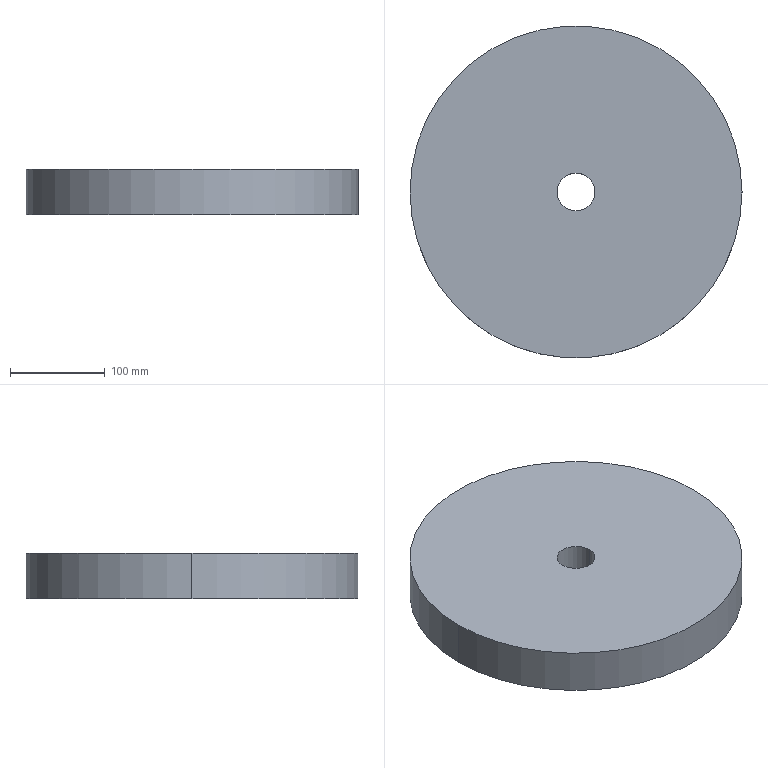Part | STEP file | 1 solid | 6 faces | box 350 x 350 x 48 mm | volume 4557823 mm3 | cylinder 4 | plane 2 | commonest cylinder face diameters 40 x2 350 x2
STEP:
#1=CARTESIAN_POINT('',(0.,0.,0.));
#2=DIRECTION('',(0.,0.,1.));
#3=DIRECTION('',(1.,0.,0.));
#4=AXIS2_PLACEMENT_3D('',#1,#2,#3);
#5=CARTESIAN_POINT('',(175.,0.,0.));
#6=VERTEX_POINT('',#5);
#7=CARTESIAN_POINT('',(-175.,0.,0.));
#8=VERTEX_POINT('',#7);
#9=CARTESIAN_POINT('',(0.,0.,0.));
#10=DIRECTION('',(0.,0.,1.));
#11=DIRECTION('',(1.,0.,0.));
#12=AXIS2_PLACEMENT_3D('',#9,#10,#11);
#13=CIRCLE('',#12,175.);
#14=CARTESIAN_POINT('',(0.,0.,0.));
#15=DIRECTION('',(0.,0.,1.));
#16=DIRECTION('',(1.,0.,0.));
#17=AXIS2_PLACEMENT_3D('',#14,#15,#16);
#18=CYLINDRICAL_SURFACE('',#17,175.);
#19=CARTESIAN_POINT('',(0.,0.));
#20=DIRECTION('',(1.,0.));
#21=VECTOR('',#20,1.);
#22=LINE('',#19,#21);
#23=(GEOMETRIC_REPRESENTATION_CONTEXT(2)PARAMETRIC_REPRESENTATION_CONTEXT()REPRESENTATION_CONTEXT('',''));
#24=DEFINITIONAL_REPRESENTATION('',(#22),#23);
#25=PCURVE('',#18,#24);
#26=CARTESIAN_POINT('',(0.,0.,0.));
#27=DIRECTION('',(0.,0.,1.));
#28=DIRECTION('',(1.,0.,0.));
#29=AXIS2_PLACEMENT_3D('',#26,#27,#28);
#30=PLANE('',#29);
#31=CARTESIAN_POINT('',(0.,0.));
#32=DIRECTION('',(1.,0.));
#33=AXIS2_PLACEMENT_2D('',#31,#32);
#34=CIRCLE('',#33,175.);
#35=(GEOMETRIC_REPRESENTATION_CONTEXT(2)PARAMETRIC_REPRESENTATION_CONTEXT()REPRESENTATION_CONTEXT('',''));
#36=DEFINITIONAL_REPRESENTATION('',(#34),#35);
#37=PCURVE('',#30,#36);
#38=SURFACE_CURVE('',#13,(#25,#37),.PCURVE_S1.);
#39=EDGE_CURVE('',#6,#8,#38,.T.);
#40=ORIENTED_EDGE('',*,*,#39,.T.);
#41=CARTESIAN_POINT('',(-175.,0.,48.));
#42=VERTEX_POINT('',#41);
#43=CARTESIAN_POINT('',(-175.,0.,0.));
#44=DIRECTION('',(0.,0.,1.));
#45=VECTOR('',#44,1.);
#46=LINE('',#43,#45);
#47=CARTESIAN_POINT('',(3.142,0.));
#48=DIRECTION('',(0.,1.));
#49=VECTOR('',#48,1.);
#50=LINE('',#47,#49);
#51=(GEOMETRIC_REPRESENTATION_CONTEXT(2)PARAMETRIC_REPRESENTATION_CONTEXT()REPRESENTATION_CONTEXT('',''));
#52=DEFINITIONAL_REPRESENTATION('',(#50),#51);
#53=PCURVE('',#18,#52);
#54=CARTESIAN_POINT('',(0.,0.,0.));
#55=DIRECTION('',(0.,0.,1.));
#56=DIRECTION('',(1.,0.,0.));
#57=AXIS2_PLACEMENT_3D('',#54,#55,#56);
#58=CYLINDRICAL_SURFACE('',#57,175.);
#59=CARTESIAN_POINT('',(3.142,0.));
#60=DIRECTION('',(0.,1.));
#61=VECTOR('',#60,1.);
#62=LINE('',#59,#61);
#63=(GEOMETRIC_REPRESENTATION_CONTEXT(2)PARAMETRIC_REPRESENTATION_CONTEXT()REPRESENTATION_CONTEXT('',''));
#64=DEFINITIONAL_REPRESENTATION('',(#62),#63);
#65=PCURVE('',#58,#64);
#66=SURFACE_CURVE('',#46,(#53,#65),.PCURVE_S1.);
#67=EDGE_CURVE('',#8,#42,#66,.T.);
#68=ORIENTED_EDGE('',*,*,#67,.T.);
#69=CARTESIAN_POINT('',(175.,0.,48.));
#70=VERTEX_POINT('',#69);
#71=CARTESIAN_POINT('',(0.,0.,48.));
#72=DIRECTION('',(0.,0.,1.));
#73=DIRECTION('',(1.,0.,0.));
#74=AXIS2_PLACEMENT_3D('',#71,#72,#73);
#75=CIRCLE('',#74,175.);
#76=CARTESIAN_POINT('',(0.,48.));
#77=DIRECTION('',(1.,0.));
#78=VECTOR('',#77,1.);
#79=LINE('',#76,#78);
#80=(GEOMETRIC_REPRESENTATION_CONTEXT(2)PARAMETRIC_REPRESENTATION_CONTEXT()REPRESENTATION_CONTEXT('',''));
#81=DEFINITIONAL_REPRESENTATION('',(#79),#80);
#82=PCURVE('',#18,#81);
#83=CARTESIAN_POINT('',(0.,0.,48.));
#84=DIRECTION('',(0.,0.,1.));
#85=DIRECTION('',(1.,0.,0.));
#86=AXIS2_PLACEMENT_3D('',#83,#84,#85);
#87=PLANE('',#86);
#88=CARTESIAN_POINT('',(0.,0.));
#89=DIRECTION('',(1.,0.));
#90=AXIS2_PLACEMENT_2D('',#88,#89);
#91=CIRCLE('',#90,175.);
#92=(GEOMETRIC_REPRESENTATION_CONTEXT(2)PARAMETRIC_REPRESENTATION_CONTEXT()REPRESENTATION_CONTEXT('',''));
#93=DEFINITIONAL_REPRESENTATION('',(#91),#92);
#94=PCURVE('',#87,#93);
#95=SURFACE_CURVE('',#75,(#82,#94),.PCURVE_S1.);
#96=EDGE_CURVE('',#70,#42,#95,.T.);
#97=ORIENTED_EDGE('',*,*,#96,.F.);
#98=CARTESIAN_POINT('',(175.,0.,0.));
#99=DIRECTION('',(0.,0.,1.));
#100=VECTOR('',#99,1.);
#101=LINE('',#98,#100);
#102=CARTESIAN_POINT('',(0.,0.));
#103=DIRECTION('',(0.,1.));
#104=VECTOR('',#103,1.);
#105=LINE('',#102,#104);
#106=(GEOMETRIC_REPRESENTATION_CONTEXT(2)PARAMETRIC_REPRESENTATION_CONTEXT()REPRESENTATION_CONTEXT('',''));
#107=DEFINITIONAL_REPRESENTATION('',(#105),#106);
#108=PCURVE('',#18,#107);
#109=CARTESIAN_POINT('',(6.283,0.));
#110=DIRECTION('',(0.,1.));
#111=VECTOR('',#110,1.);
#112=LINE('',#109,#111);
#113=(GEOMETRIC_REPRESENTATION_CONTEXT(2)PARAMETRIC_REPRESENTATION_CONTEXT()REPRESENTATION_CONTEXT('',''));
#114=DEFINITIONAL_REPRESENTATION('',(#112),#113);
#115=PCURVE('',#58,#114);
#116=SURFACE_CURVE('',#101,(#108,#115),.PCURVE_S1.);
#117=EDGE_CURVE('',#6,#70,#116,.T.);
#118=ORIENTED_EDGE('',*,*,#117,.F.);
#119=EDGE_LOOP('',(#40,#68,#97,#118));
#120=FACE_BOUND('',#119,.T.);
#121=ADVANCED_FACE('',(#120),#18,.T.);
#122=CARTESIAN_POINT('',(-20.,0.,48.));
#123=VERTEX_POINT('',#122);
#124=CARTESIAN_POINT('',(-20.,0.,0.));
#125=VERTEX_POINT('',#124);
#126=CARTESIAN_POINT('',(-20.,0.,48.));
#127=DIRECTION('',(0.,0.,-1.));
#128=VECTOR('',#127,1.);
#129=LINE('',#126,#128);
#130=CARTESIAN_POINT('',(0.,0.,48.));
#131=DIRECTION('',(0.,0.,-1.));
#132=DIRECTION('',(-1.,0.,0.));
#133=AXIS2_PLACEMENT_3D('',#130,#131,#132);
#134=CYLINDRICAL_SURFACE('',#133,20.);
#135=CARTESIAN_POINT('',(6.283,0.));
#136=DIRECTION('',(0.,1.));
#137=VECTOR('',#136,1.);
#138=LINE('',#135,#137);
#139=(GEOMETRIC_REPRESENTATION_CONTEXT(2)PARAMETRIC_REPRESENTATION_CONTEXT()REPRESENTATION_CONTEXT('',''));
#140=DEFINITIONAL_REPRESENTATION('',(#138),#139);
#141=PCURVE('',#134,#140);
#142=CARTESIAN_POINT('',(0.,0.,48.));
#143=DIRECTION('',(0.,0.,-1.));
#144=DIRECTION('',(-1.,0.,0.));
#145=AXIS2_PLACEMENT_3D('',#142,#143,#144);
#146=CYLINDRICAL_SURFACE('',#145,20.);
#147=CARTESIAN_POINT('',(0.,0.));
#148=DIRECTION('',(0.,1.));
#149=VECTOR('',#148,1.);
#150=LINE('',#147,#149);
#151=(GEOMETRIC_REPRESENTATION_CONTEXT(2)PARAMETRIC_REPRESENTATION_CONTEXT()REPRESENTATION_CONTEXT('',''));
#152=DEFINITIONAL_REPRESENTATION('',(#150),#151);
#153=PCURVE('',#146,#152);
#154=SURFACE_CURVE('',#129,(#141,#153),.PCURVE_S1.);
#155=EDGE_CURVE('',#123,#125,#154,.T.);
#156=ORIENTED_EDGE('',*,*,#155,.T.);
#157=CARTESIAN_POINT('',(20.,0.,0.));
#158=VERTEX_POINT('',#157);
#159=CARTESIAN_POINT('',(0.,0.,0.));
#160=DIRECTION('',(0.,0.,1.));
#161=DIRECTION('',(-1.,0.,0.));
#162=AXIS2_PLACEMENT_3D('',#159,#160,#161);
#163=CIRCLE('',#162,20.);
#164=CARTESIAN_POINT('',(6.283,48.));
#165=DIRECTION('',(-1.,0.));
#166=VECTOR('',#165,1.);
#167=LINE('',#164,#166);
#168=(GEOMETRIC_REPRESENTATION_CONTEXT(2)PARAMETRIC_REPRESENTATION_CONTEXT()REPRESENTATION_CONTEXT('',''));
#169=DEFINITIONAL_REPRESENTATION('',(#167),#168);
#170=PCURVE('',#134,#169);
#171=CARTESIAN_POINT('',(0.,0.));
#172=DIRECTION('',(-1.,0.));
#173=AXIS2_PLACEMENT_2D('',#171,#172);
#174=CIRCLE('',#173,20.);
#175=(GEOMETRIC_REPRESENTATION_CONTEXT(2)PARAMETRIC_REPRESENTATION_CONTEXT()REPRESENTATION_CONTEXT('',''));
#176=DEFINITIONAL_REPRESENTATION('',(#174),#175);
#177=PCURVE('',#30,#176);
#178=SURFACE_CURVE('',#163,(#170,#177),.PCURVE_S1.);
#179=EDGE_CURVE('',#125,#158,#178,.T.);
#180=ORIENTED_EDGE('',*,*,#179,.T.);
#181=CARTESIAN_POINT('',(20.,0.,48.));
#182=VERTEX_POINT('',#181);
#183=CARTESIAN_POINT('',(20.,0.,48.));
#184=DIRECTION('',(0.,0.,-1.));
#185=VECTOR('',#184,1.);
#186=LINE('',#183,#185);
#187=CARTESIAN_POINT('',(3.142,0.));
#188=DIRECTION('',(0.,1.));
#189=VECTOR('',#188,1.);
#190=LINE('',#187,#189);
#191=(GEOMETRIC_REPRESENTATION_CONTEXT(2)PARAMETRIC_REPRESENTATION_CONTEXT()REPRESENTATION_CONTEXT('',''));
#192=DEFINITIONAL_REPRESENTATION('',(#190),#191);
#193=PCURVE('',#134,#192);
#194=CARTESIAN_POINT('',(3.142,0.));
#195=DIRECTION('',(0.,1.));
#196=VECTOR('',#195,1.);
#197=LINE('',#194,#196);
#198=(GEOMETRIC_REPRESENTATION_CONTEXT(2)PARAMETRIC_REPRESENTATION_CONTEXT()REPRESENTATION_CONTEXT('',''));
#199=DEFINITIONAL_REPRESENTATION('',(#197),#198);
#200=PCURVE('',#146,#199);
#201=SURFACE_CURVE('',#186,(#193,#200),.PCURVE_S1.);
#202=EDGE_CURVE('',#182,#158,#201,.T.);
#203=ORIENTED_EDGE('',*,*,#202,.F.);
#204=CARTESIAN_POINT('',(0.,0.,48.));
#205=DIRECTION('',(0.,0.,-1.));
#206=DIRECTION('',(-1.,0.,0.));
#207=AXIS2_PLACEMENT_3D('',#204,#205,#206);
#208=CIRCLE('',#207,20.);
#209=CARTESIAN_POINT('',(0.,0.));
#210=DIRECTION('',(1.,0.));
#211=VECTOR('',#210,1.);
#212=LINE('',#209,#211);
#213=(GEOMETRIC_REPRESENTATION_CONTEXT(2)PARAMETRIC_REPRESENTATION_CONTEXT()REPRESENTATION_CONTEXT('',''));
#214=DEFINITIONAL_REPRESENTATION('',(#212),#213);
#215=PCURVE('',#134,#214);
#216=CARTESIAN_POINT('',(-20.,0.));
#217=CARTESIAN_POINT('',(-20.,34.641));
#218=CARTESIAN_POINT('',(10.,17.321));
#219=CARTESIAN_POINT('',(40.,0.));
#220=CARTESIAN_POINT('',(10.,-17.321));
#221=CARTESIAN_POINT('',(-20.,-34.641));
#222=CARTESIAN_POINT('',(-20.,0.));
#223=(BOUNDED_CURVE()B_SPLINE_CURVE(2,(#216,#217,#218,#219,#220,#221,#222),.UNSPECIFIED.,.T.,.F.)B_SPLINE_CURVE_WITH_KNOTS((1,2,2,2,2,1),(-2.094,0.,2.094,4.189,6.283,8.378),.UNSPECIFIED.)CURVE()GEOMETRIC_REPRESENTATION_ITEM()RATIONAL_B_SPLINE_CURVE((1.,0.5,1.,0.5,1.,0.5,1.))REPRESENTATION_ITEM(''));
#224=(GEOMETRIC_REPRESENTATION_CONTEXT(2)PARAMETRIC_REPRESENTATION_CONTEXT()REPRESENTATION_CONTEXT('',''));
#225=DEFINITIONAL_REPRESENTATION('',(#223),#224);
#226=PCURVE('',#87,#225);
#227=SURFACE_CURVE('',#208,(#215,#226),.PCURVE_S1.);
#228=EDGE_CURVE('',#182,#123,#227,.T.);
#229=ORIENTED_EDGE('',*,*,#228,.T.);
#230=EDGE_LOOP('',(#156,#180,#203,#229));
#231=FACE_BOUND('',#230,.F.);
#232=ADVANCED_FACE('',(#231),#134,.F.);
#233=ORIENTED_EDGE('',*,*,#96,.T.);
#234=CARTESIAN_POINT('',(0.,0.,48.));
#235=DIRECTION('',(0.,0.,1.));
#236=DIRECTION('',(1.,0.,0.));
#237=AXIS2_PLACEMENT_3D('',#234,#235,#236);
#238=CIRCLE('',#237,175.);
#239=CARTESIAN_POINT('',(0.,0.));
#240=DIRECTION('',(1.,0.));
#241=AXIS2_PLACEMENT_2D('',#239,#240);
#242=CIRCLE('',#241,175.);
#243=(GEOMETRIC_REPRESENTATION_CONTEXT(2)PARAMETRIC_REPRESENTATION_CONTEXT()REPRESENTATION_CONTEXT('',''));
#244=DEFINITIONAL_REPRESENTATION('',(#242),#243);
#245=PCURVE('',#87,#244);
#246=CARTESIAN_POINT('',(0.,48.));
#247=DIRECTION('',(1.,0.));
#248=VECTOR('',#247,1.);
#249=LINE('',#246,#248);
#250=(GEOMETRIC_REPRESENTATION_CONTEXT(2)PARAMETRIC_REPRESENTATION_CONTEXT()REPRESENTATION_CONTEXT('',''));
#251=DEFINITIONAL_REPRESENTATION('',(#249),#250);
#252=PCURVE('',#58,#251);
#253=SURFACE_CURVE('',#238,(#245,#252),.PCURVE_S1.);
#254=EDGE_CURVE('',#42,#70,#253,.T.);
#255=ORIENTED_EDGE('',*,*,#254,.T.);
#256=EDGE_LOOP('',(#233,#255));
#257=FACE_BOUND('',#256,.T.);
#258=CARTESIAN_POINT('',(0.,0.,48.));
#259=DIRECTION('',(0.,0.,-1.));
#260=DIRECTION('',(-1.,0.,0.));
#261=AXIS2_PLACEMENT_3D('',#258,#259,#260);
#262=CIRCLE('',#261,20.);
#263=CARTESIAN_POINT('',(-20.,0.));
#264=CARTESIAN_POINT('',(-20.,34.641));
#265=CARTESIAN_POINT('',(10.,17.321));
#266=CARTESIAN_POINT('',(40.,0.));
#267=CARTESIAN_POINT('',(10.,-17.321));
#268=CARTESIAN_POINT('',(-20.,-34.641));
#269=CARTESIAN_POINT('',(-20.,0.));
#270=(BOUNDED_CURVE()B_SPLINE_CURVE(2,(#263,#264,#265,#266,#267,#268,#269),.UNSPECIFIED.,.T.,.F.)B_SPLINE_CURVE_WITH_KNOTS((1,2,2,2,2,1),(-2.094,0.,2.094,4.189,6.283,8.378),.UNSPECIFIED.)CURVE()GEOMETRIC_REPRESENTATION_ITEM()RATIONAL_B_SPLINE_CURVE((1.,0.5,1.,0.5,1.,0.5,1.))REPRESENTATION_ITEM(''));
#271=(GEOMETRIC_REPRESENTATION_CONTEXT(2)PARAMETRIC_REPRESENTATION_CONTEXT()REPRESENTATION_CONTEXT('',''));
#272=DEFINITIONAL_REPRESENTATION('',(#270),#271);
#273=PCURVE('',#87,#272);
#274=CARTESIAN_POINT('',(0.,0.));
#275=DIRECTION('',(1.,0.));
#276=VECTOR('',#275,1.);
#277=LINE('',#274,#276);
#278=(GEOMETRIC_REPRESENTATION_CONTEXT(2)PARAMETRIC_REPRESENTATION_CONTEXT()REPRESENTATION_CONTEXT('',''));
#279=DEFINITIONAL_REPRESENTATION('',(#277),#278);
#280=PCURVE('',#146,#279);
#281=SURFACE_CURVE('',#262,(#273,#280),.PCURVE_S1.);
#282=EDGE_CURVE('',#123,#182,#281,.T.);
#283=ORIENTED_EDGE('',*,*,#282,.T.);
#284=ORIENTED_EDGE('',*,*,#228,.T.);
#285=EDGE_LOOP('',(#283,#284));
#286=FACE_BOUND('',#285,.T.);
#287=ADVANCED_FACE('',(#257,#286),#87,.T.);
#288=ORIENTED_EDGE('',*,*,#67,.F.);
#289=CARTESIAN_POINT('',(0.,0.,0.));
#290=DIRECTION('',(0.,0.,1.));
#291=DIRECTION('',(1.,0.,0.));
#292=AXIS2_PLACEMENT_3D('',#289,#290,#291);
#293=CIRCLE('',#292,175.);
#294=CARTESIAN_POINT('',(0.,0.));
#295=DIRECTION('',(1.,0.));
#296=VECTOR('',#295,1.);
#297=LINE('',#294,#296);
#298=(GEOMETRIC_REPRESENTATION_CONTEXT(2)PARAMETRIC_REPRESENTATION_CONTEXT()REPRESENTATION_CONTEXT('',''));
#299=DEFINITIONAL_REPRESENTATION('',(#297),#298);
#300=PCURVE('',#58,#299);
#301=CARTESIAN_POINT('',(0.,0.));
#302=DIRECTION('',(1.,0.));
#303=AXIS2_PLACEMENT_2D('',#301,#302);
#304=CIRCLE('',#303,175.);
#305=(GEOMETRIC_REPRESENTATION_CONTEXT(2)PARAMETRIC_REPRESENTATION_CONTEXT()REPRESENTATION_CONTEXT('',''));
#306=DEFINITIONAL_REPRESENTATION('',(#304),#305);
#307=PCURVE('',#30,#306);
#308=SURFACE_CURVE('',#293,(#300,#307),.PCURVE_S1.);
#309=EDGE_CURVE('',#8,#6,#308,.T.);
#310=ORIENTED_EDGE('',*,*,#309,.T.);
#311=ORIENTED_EDGE('',*,*,#117,.T.);
#312=ORIENTED_EDGE('',*,*,#254,.F.);
#313=EDGE_LOOP('',(#288,#310,#311,#312));
#314=FACE_BOUND('',#313,.T.);
#315=ADVANCED_FACE('',(#314),#58,.T.);
#316=CARTESIAN_POINT('',(0.,0.,0.));
#317=DIRECTION('',(0.,0.,1.));
#318=DIRECTION('',(-1.,0.,0.));
#319=AXIS2_PLACEMENT_3D('',#316,#317,#318);
#320=CIRCLE('',#319,20.);
#321=CARTESIAN_POINT('',(6.283,48.));
#322=DIRECTION('',(-1.,0.));
#323=VECTOR('',#322,1.);
#324=LINE('',#321,#323);
#325=(GEOMETRIC_REPRESENTATION_CONTEXT(2)PARAMETRIC_REPRESENTATION_CONTEXT()REPRESENTATION_CONTEXT('',''));
#326=DEFINITIONAL_REPRESENTATION('',(#324),#325);
#327=PCURVE('',#146,#326);
#328=CARTESIAN_POINT('',(0.,0.));
#329=DIRECTION('',(-1.,0.));
#330=AXIS2_PLACEMENT_2D('',#328,#329);
#331=CIRCLE('',#330,20.);
#332=(GEOMETRIC_REPRESENTATION_CONTEXT(2)PARAMETRIC_REPRESENTATION_CONTEXT()REPRESENTATION_CONTEXT('',''));
#333=DEFINITIONAL_REPRESENTATION('',(#331),#332);
#334=PCURVE('',#30,#333);
#335=SURFACE_CURVE('',#320,(#327,#334),.PCURVE_S1.);
#336=EDGE_CURVE('',#158,#125,#335,.T.);
#337=ORIENTED_EDGE('',*,*,#336,.T.);
#338=ORIENTED_EDGE('',*,*,#155,.F.);
#339=ORIENTED_EDGE('',*,*,#282,.T.);
#340=ORIENTED_EDGE('',*,*,#202,.T.);
#341=EDGE_LOOP('',(#337,#338,#339,#340));
#342=FACE_BOUND('',#341,.F.);
#343=ADVANCED_FACE('',(#342),#146,.F.);
#344=ORIENTED_EDGE('',*,*,#39,.F.);
#345=ORIENTED_EDGE('',*,*,#309,.F.);
#346=EDGE_LOOP('',(#344,#345));
#347=FACE_BOUND('',#346,.T.);
#348=ORIENTED_EDGE('',*,*,#179,.T.);
#349=ORIENTED_EDGE('',*,*,#336,.T.);
#350=EDGE_LOOP('',(#348,#349));
#351=FACE_BOUND('',#350,.T.);
#352=ADVANCED_FACE('',(#347,#351),#30,.F.);
#353=CLOSED_SHELL('',(#121,#232,#287,#315,#343,#352));
#354=MANIFOLD_SOLID_BREP('',#353);
#355=(LENGTH_UNIT()NAMED_UNIT(*)SI_UNIT(.MILLI.,.METRE.));
#356=UNCERTAINTY_MEASURE_WITH_UNIT(LENGTH_MEASURE(0.0000001),#355,'','');
#357=(NAMED_UNIT(*)PLANE_ANGLE_UNIT()SI_UNIT($,.RADIAN.));
#358=(NAMED_UNIT(*)SI_UNIT($,.STERADIAN.)SOLID_ANGLE_UNIT());
#359=(GEOMETRIC_REPRESENTATION_CONTEXT(3)GLOBAL_UNCERTAINTY_ASSIGNED_CONTEXT((#356))GLOBAL_UNIT_ASSIGNED_CONTEXT((#355,#357,#358))REPRESENTATION_CONTEXT('',''));
#360=ADVANCED_BREP_SHAPE_REPRESENTATION('',(#4,#354),#359);